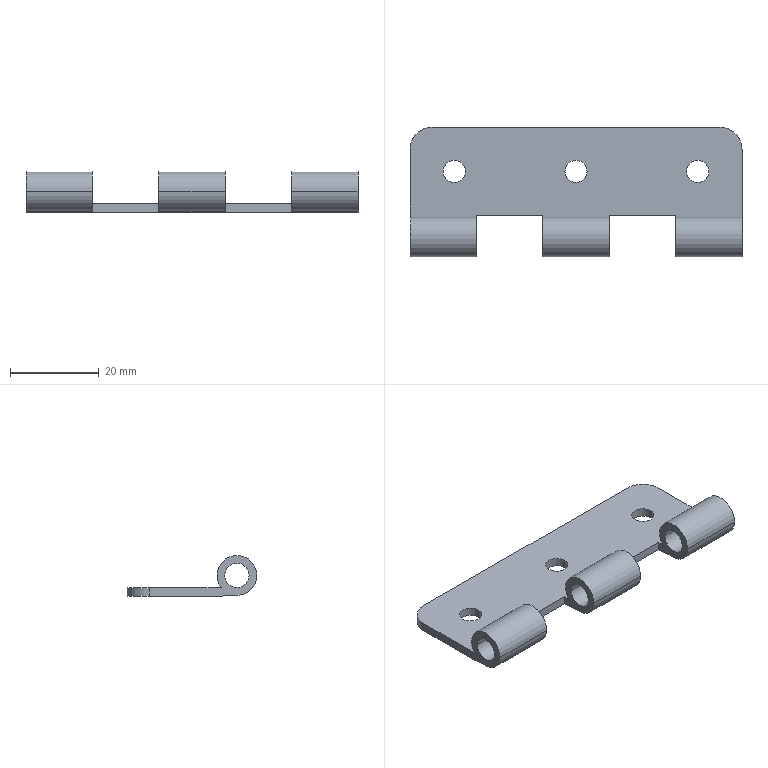Part | SolidWorks | features Extrusion 1, Fillet 1, ICE 1, LPattern 1 | 1 solid | 37 faces | box 75 x 29.3 x 9.25 mm | volume 4864 mm3 | cylinder 23 | plane 14 | commonest cylinder face diameters 9 x9 5 x6 5.5 x6 10 x2
STEP:
#1=CARTESIAN_POINT('',(75.,-22.05,4.75));
#2=VERTEX_POINT('',#1);
#3=CARTESIAN_POINT('',(75.,-27.55,4.75));
#4=VERTEX_POINT('',#3);
#5=CARTESIAN_POINT('',(75.,-24.8,4.75));
#6=DIRECTION('',(-1.,0.,0.));
#7=DIRECTION('',(0.,-1.,0.));
#8=AXIS2_PLACEMENT_3D('',#5,#6,#7);
#9=CIRCLE('',#8,2.75);
#10=EDGE_CURVE('',#2,#4,#9,.T.);
#11=ORIENTED_EDGE('',*,*,#10,.F.);
#12=CARTESIAN_POINT('',(60.,-22.05,4.75));
#13=VERTEX_POINT('',#12);
#14=CARTESIAN_POINT('',(75.,-22.05,4.75));
#15=DIRECTION('',(-1.,0.,0.));
#16=VECTOR('',#15,1000.);
#17=LINE('',#14,#16);
#18=EDGE_CURVE('',#2,#13,#17,.T.);
#19=ORIENTED_EDGE('',*,*,#18,.T.);
#20=CARTESIAN_POINT('',(60.,-27.55,4.75));
#21=VERTEX_POINT('',#20);
#22=CARTESIAN_POINT('',(60.,-24.8,4.75));
#23=DIRECTION('',(-1.,0.,0.));
#24=DIRECTION('',(0.,-1.,0.));
#25=AXIS2_PLACEMENT_3D('',#22,#23,#24);
#26=CIRCLE('',#25,2.75);
#27=EDGE_CURVE('',#13,#21,#26,.T.);
#28=ORIENTED_EDGE('',*,*,#27,.T.);
#29=CARTESIAN_POINT('',(75.,-27.55,4.75));
#30=DIRECTION('',(-1.,0.,0.));
#31=VECTOR('',#30,1000.);
#32=LINE('',#29,#31);
#33=EDGE_CURVE('',#4,#21,#32,.T.);
#34=ORIENTED_EDGE('',*,*,#33,.F.);
#35=EDGE_LOOP('',(#11,#19,#28,#34));
#36=FACE_OUTER_BOUND('',#35,.T.);
#37=CARTESIAN_POINT('',(75.,-24.8,4.75));
#38=DIRECTION('',(-1.,0.,0.));
#39=DIRECTION('',(0.,-1.,0.));
#40=AXIS2_PLACEMENT_3D('',#37,#38,#39);
#41=CYLINDRICAL_SURFACE('',#40,2.75);
#42=ADVANCED_FACE('',(#36),#41,.F.);
#43=CARTESIAN_POINT('',(75.,-29.3,4.75));
#44=VERTEX_POINT('',#43);
#45=CARTESIAN_POINT('',(75.,-20.3,4.75));
#46=VERTEX_POINT('',#45);
#47=CARTESIAN_POINT('',(75.,-24.8,4.75));
#48=DIRECTION('',(-1.,0.,0.));
#49=DIRECTION('',(0.,-1.,0.));
#50=AXIS2_PLACEMENT_3D('',#47,#48,#49);
#51=CIRCLE('',#50,4.5);
#52=EDGE_CURVE('',#44,#46,#51,.T.);
#53=ORIENTED_EDGE('',*,*,#52,.T.);
#54=CARTESIAN_POINT('',(60.,-20.3,4.75));
#55=VERTEX_POINT('',#54);
#56=CARTESIAN_POINT('',(75.,-20.3,4.75));
#57=DIRECTION('',(-1.,0.,0.));
#58=VECTOR('',#57,1000.);
#59=LINE('',#56,#58);
#60=EDGE_CURVE('',#46,#55,#59,.T.);
#61=ORIENTED_EDGE('',*,*,#60,.T.);
#62=CARTESIAN_POINT('',(60.,-29.3,4.75));
#63=VERTEX_POINT('',#62);
#64=CARTESIAN_POINT('',(60.,-24.8,4.75));
#65=DIRECTION('',(-1.,0.,0.));
#66=DIRECTION('',(0.,-1.,0.));
#67=AXIS2_PLACEMENT_3D('',#64,#65,#66);
#68=CIRCLE('',#67,4.5);
#69=EDGE_CURVE('',#63,#55,#68,.T.);
#70=ORIENTED_EDGE('',*,*,#69,.F.);
#71=CARTESIAN_POINT('',(75.,-29.3,4.75));
#72=DIRECTION('',(-1.,0.,0.));
#73=VECTOR('',#72,1000.);
#74=LINE('',#71,#73);
#75=EDGE_CURVE('',#44,#63,#74,.T.);
#76=ORIENTED_EDGE('',*,*,#75,.F.);
#77=EDGE_LOOP('',(#53,#61,#70,#76));
#78=FACE_OUTER_BOUND('',#77,.T.);
#79=CARTESIAN_POINT('',(75.,-24.8,4.75));
#80=DIRECTION('',(-1.,0.,0.));
#81=DIRECTION('',(0.,-1.,0.));
#82=AXIS2_PLACEMENT_3D('',#79,#80,#81);
#83=CYLINDRICAL_SURFACE('',#82,4.5);
#84=ADVANCED_FACE('',(#78),#83,.T.);
#85=CARTESIAN_POINT('',(75.,-25.029,0.2558));
#86=VERTEX_POINT('',#85);
#87=CARTESIAN_POINT('',(75.,-24.8,4.75));
#88=DIRECTION('',(-1.,0.,0.));
#89=DIRECTION('',(0.,-1.,0.));
#90=AXIS2_PLACEMENT_3D('',#87,#88,#89);
#91=CIRCLE('',#90,4.5);
#92=EDGE_CURVE('',#86,#44,#91,.T.);
#93=ORIENTED_EDGE('',*,*,#92,.T.);
#94=ORIENTED_EDGE('',*,*,#75,.T.);
#95=CARTESIAN_POINT('',(60.,-25.029,0.2558));
#96=VERTEX_POINT('',#95);
#97=CARTESIAN_POINT('',(60.,-24.8,4.75));
#98=DIRECTION('',(-1.,0.,0.));
#99=DIRECTION('',(0.,-1.,0.));
#100=AXIS2_PLACEMENT_3D('',#97,#98,#99);
#101=CIRCLE('',#100,4.5);
#102=EDGE_CURVE('',#96,#63,#101,.T.);
#103=ORIENTED_EDGE('',*,*,#102,.F.);
#104=CARTESIAN_POINT('',(75.,-25.029,0.2558));
#105=DIRECTION('',(-1.,0.,0.));
#106=VECTOR('',#105,1000.);
#107=LINE('',#104,#106);
#108=EDGE_CURVE('',#86,#96,#107,.T.);
#109=ORIENTED_EDGE('',*,*,#108,.F.);
#110=EDGE_LOOP('',(#93,#94,#103,#109));
#111=FACE_OUTER_BOUND('',#110,.T.);
#112=CARTESIAN_POINT('',(75.,-24.8,4.75));
#113=DIRECTION('',(-1.,0.,0.));
#114=DIRECTION('',(0.,-1.,0.));
#115=AXIS2_PLACEMENT_3D('',#112,#113,#114);
#116=CYLINDRICAL_SURFACE('',#115,4.5);
#117=ADVANCED_FACE('',(#111),#116,.T.);
#118=CARTESIAN_POINT('',(45.,-22.05,4.75));
#119=VERTEX_POINT('',#118);
#120=CARTESIAN_POINT('',(45.,-27.55,4.75));
#121=VERTEX_POINT('',#120);
#122=CARTESIAN_POINT('',(45.,-24.8,4.75));
#123=DIRECTION('',(-1.,0.,0.));
#124=DIRECTION('',(0.,-1.,0.));
#125=AXIS2_PLACEMENT_3D('',#122,#123,#124);
#126=CIRCLE('',#125,2.75);
#127=EDGE_CURVE('',#119,#121,#126,.T.);
#128=ORIENTED_EDGE('',*,*,#127,.F.);
#129=CARTESIAN_POINT('',(30.,-22.05,4.75));
#130=VERTEX_POINT('',#129);
#131=CARTESIAN_POINT('',(45.,-22.05,4.75));
#132=DIRECTION('',(-1.,0.,0.));
#133=VECTOR('',#132,1000.);
#134=LINE('',#131,#133);
#135=EDGE_CURVE('',#119,#130,#134,.T.);
#136=ORIENTED_EDGE('',*,*,#135,.T.);
#137=CARTESIAN_POINT('',(30.,-27.55,4.75));
#138=VERTEX_POINT('',#137);
#139=CARTESIAN_POINT('',(30.,-24.8,4.75));
#140=DIRECTION('',(-1.,0.,0.));
#141=DIRECTION('',(0.,-1.,0.));
#142=AXIS2_PLACEMENT_3D('',#139,#140,#141);
#143=CIRCLE('',#142,2.75);
#144=EDGE_CURVE('',#130,#138,#143,.T.);
#145=ORIENTED_EDGE('',*,*,#144,.T.);
#146=CARTESIAN_POINT('',(45.,-27.55,4.75));
#147=DIRECTION('',(-1.,0.,0.));
#148=VECTOR('',#147,1000.);
#149=LINE('',#146,#148);
#150=EDGE_CURVE('',#121,#138,#149,.T.);
#151=ORIENTED_EDGE('',*,*,#150,.F.);
#152=EDGE_LOOP('',(#128,#136,#145,#151));
#153=FACE_OUTER_BOUND('',#152,.T.);
#154=CARTESIAN_POINT('',(45.,-24.8,4.75));
#155=DIRECTION('',(-1.,0.,0.));
#156=DIRECTION('',(0.,-1.,0.));
#157=AXIS2_PLACEMENT_3D('',#154,#155,#156);
#158=CYLINDRICAL_SURFACE('',#157,2.75);
#159=ADVANCED_FACE('',(#153),#158,.F.);
#160=CARTESIAN_POINT('',(45.,-29.3,4.75));
#161=VERTEX_POINT('',#160);
#162=CARTESIAN_POINT('',(45.,-20.3,4.75));
#163=VERTEX_POINT('',#162);
#164=CARTESIAN_POINT('',(45.,-24.8,4.75));
#165=DIRECTION('',(-1.,0.,0.));
#166=DIRECTION('',(0.,-1.,0.));
#167=AXIS2_PLACEMENT_3D('',#164,#165,#166);
#168=CIRCLE('',#167,4.5);
#169=EDGE_CURVE('',#161,#163,#168,.T.);
#170=ORIENTED_EDGE('',*,*,#169,.T.);
#171=CARTESIAN_POINT('',(30.,-20.3,4.75));
#172=VERTEX_POINT('',#171);
#173=CARTESIAN_POINT('',(45.,-20.3,4.75));
#174=DIRECTION('',(-1.,0.,0.));
#175=VECTOR('',#174,1000.);
#176=LINE('',#173,#175);
#177=EDGE_CURVE('',#163,#172,#176,.T.);
#178=ORIENTED_EDGE('',*,*,#177,.T.);
#179=CARTESIAN_POINT('',(30.,-29.3,4.75));
#180=VERTEX_POINT('',#179);
#181=CARTESIAN_POINT('',(30.,-24.8,4.75));
#182=DIRECTION('',(-1.,0.,0.));
#183=DIRECTION('',(0.,-1.,0.));
#184=AXIS2_PLACEMENT_3D('',#181,#182,#183);
#185=CIRCLE('',#184,4.5);
#186=EDGE_CURVE('',#180,#172,#185,.T.);
#187=ORIENTED_EDGE('',*,*,#186,.F.);
#188=CARTESIAN_POINT('',(45.,-29.3,4.75));
#189=DIRECTION('',(-1.,0.,0.));
#190=VECTOR('',#189,1000.);
#191=LINE('',#188,#190);
#192=EDGE_CURVE('',#161,#180,#191,.T.);
#193=ORIENTED_EDGE('',*,*,#192,.F.);
#194=EDGE_LOOP('',(#170,#178,#187,#193));
#195=FACE_OUTER_BOUND('',#194,.T.);
#196=CARTESIAN_POINT('',(45.,-24.8,4.75));
#197=DIRECTION('',(-1.,0.,0.));
#198=DIRECTION('',(0.,-1.,0.));
#199=AXIS2_PLACEMENT_3D('',#196,#197,#198);
#200=CYLINDRICAL_SURFACE('',#199,4.5);
#201=ADVANCED_FACE('',(#195),#200,.T.);
#202=CARTESIAN_POINT('',(45.,-25.029,0.2558));
#203=VERTEX_POINT('',#202);
#204=CARTESIAN_POINT('',(45.,-24.8,4.75));
#205=DIRECTION('',(-1.,0.,0.));
#206=DIRECTION('',(0.,-1.,0.));
#207=AXIS2_PLACEMENT_3D('',#204,#205,#206);
#208=CIRCLE('',#207,4.5);
#209=EDGE_CURVE('',#203,#161,#208,.T.);
#210=ORIENTED_EDGE('',*,*,#209,.T.);
#211=ORIENTED_EDGE('',*,*,#192,.T.);
#212=CARTESIAN_POINT('',(30.,-25.029,0.2558));
#213=VERTEX_POINT('',#212);
#214=CARTESIAN_POINT('',(30.,-24.8,4.75));
#215=DIRECTION('',(-1.,0.,0.));
#216=DIRECTION('',(0.,-1.,0.));
#217=AXIS2_PLACEMENT_3D('',#214,#215,#216);
#218=CIRCLE('',#217,4.5);
#219=EDGE_CURVE('',#213,#180,#218,.T.);
#220=ORIENTED_EDGE('',*,*,#219,.F.);
#221=CARTESIAN_POINT('',(45.,-25.029,0.2558));
#222=DIRECTION('',(-1.,0.,0.));
#223=VECTOR('',#222,1000.);
#224=LINE('',#221,#223);
#225=EDGE_CURVE('',#203,#213,#224,.T.);
#226=ORIENTED_EDGE('',*,*,#225,.F.);
#227=EDGE_LOOP('',(#210,#211,#220,#226));
#228=FACE_OUTER_BOUND('',#227,.T.);
#229=CARTESIAN_POINT('',(45.,-24.8,4.75));
#230=DIRECTION('',(-1.,0.,0.));
#231=DIRECTION('',(0.,-1.,0.));
#232=AXIS2_PLACEMENT_3D('',#229,#230,#231);
#233=CYLINDRICAL_SURFACE('',#232,4.5);
#234=ADVANCED_FACE('',(#228),#233,.T.);
#235=CARTESIAN_POINT('',(15.,-22.05,4.75));
#236=VERTEX_POINT('',#235);
#237=CARTESIAN_POINT('',(15.,-27.55,4.75));
#238=VERTEX_POINT('',#237);
#239=CARTESIAN_POINT('',(15.,-24.8,4.75));
#240=DIRECTION('',(-1.,0.,0.));
#241=DIRECTION('',(0.,-1.,0.));
#242=AXIS2_PLACEMENT_3D('',#239,#240,#241);
#243=CIRCLE('',#242,2.75);
#244=EDGE_CURVE('',#236,#238,#243,.T.);
#245=ORIENTED_EDGE('',*,*,#244,.F.);
#246=CARTESIAN_POINT('',(0.,-22.05,4.75));
#247=VERTEX_POINT('',#246);
#248=CARTESIAN_POINT('',(15.,-22.05,4.75));
#249=DIRECTION('',(-1.,0.,0.));
#250=VECTOR('',#249,1000.);
#251=LINE('',#248,#250);
#252=EDGE_CURVE('',#236,#247,#251,.T.);
#253=ORIENTED_EDGE('',*,*,#252,.T.);
#254=CARTESIAN_POINT('',(0.,-27.55,4.75));
#255=VERTEX_POINT('',#254);
#256=CARTESIAN_POINT('',(0.,-24.8,4.75));
#257=DIRECTION('',(-1.,0.,0.));
#258=DIRECTION('',(0.,-1.,0.));
#259=AXIS2_PLACEMENT_3D('',#256,#257,#258);
#260=CIRCLE('',#259,2.75);
#261=EDGE_CURVE('',#247,#255,#260,.T.);
#262=ORIENTED_EDGE('',*,*,#261,.T.);
#263=CARTESIAN_POINT('',(15.,-27.55,4.75));
#264=DIRECTION('',(-1.,0.,0.));
#265=VECTOR('',#264,1000.);
#266=LINE('',#263,#265);
#267=EDGE_CURVE('',#238,#255,#266,.T.);
#268=ORIENTED_EDGE('',*,*,#267,.F.);
#269=EDGE_LOOP('',(#245,#253,#262,#268));
#270=FACE_OUTER_BOUND('',#269,.T.);
#271=CARTESIAN_POINT('',(15.,-24.8,4.75));
#272=DIRECTION('',(-1.,0.,0.));
#273=DIRECTION('',(0.,-1.,0.));
#274=AXIS2_PLACEMENT_3D('',#271,#272,#273);
#275=CYLINDRICAL_SURFACE('',#274,2.75);
#276=ADVANCED_FACE('',(#270),#275,.F.);
#277=CARTESIAN_POINT('',(15.,-29.3,4.75));
#278=VERTEX_POINT('',#277);
#279=CARTESIAN_POINT('',(15.,-20.3,4.75));
#280=VERTEX_POINT('',#279);
#281=CARTESIAN_POINT('',(15.,-24.8,4.75));
#282=DIRECTION('',(-1.,0.,0.));
#283=DIRECTION('',(0.,-1.,0.));
#284=AXIS2_PLACEMENT_3D('',#281,#282,#283);
#285=CIRCLE('',#284,4.5);
#286=EDGE_CURVE('',#278,#280,#285,.T.);
#287=ORIENTED_EDGE('',*,*,#286,.T.);
#288=CARTESIAN_POINT('',(0.,-20.3,4.75));
#289=VERTEX_POINT('',#288);
#290=CARTESIAN_POINT('',(15.,-20.3,4.75));
#291=DIRECTION('',(-1.,0.,0.));
#292=VECTOR('',#291,1000.);
#293=LINE('',#290,#292);
#294=EDGE_CURVE('',#280,#289,#293,.T.);
#295=ORIENTED_EDGE('',*,*,#294,.T.);
#296=CARTESIAN_POINT('',(0.,-29.3,4.75));
#297=VERTEX_POINT('',#296);
#298=CARTESIAN_POINT('',(0.,-24.8,4.75));
#299=DIRECTION('',(-1.,0.,0.));
#300=DIRECTION('',(0.,-1.,0.));
#301=AXIS2_PLACEMENT_3D('',#298,#299,#300);
#302=CIRCLE('',#301,4.5);
#303=EDGE_CURVE('',#297,#289,#302,.T.);
#304=ORIENTED_EDGE('',*,*,#303,.F.);
#305=CARTESIAN_POINT('',(15.,-29.3,4.75));
#306=DIRECTION('',(-1.,0.,0.));
#307=VECTOR('',#306,1000.);
#308=LINE('',#305,#307);
#309=EDGE_CURVE('',#278,#297,#308,.T.);
#310=ORIENTED_EDGE('',*,*,#309,.F.);
#311=EDGE_LOOP('',(#287,#295,#304,#310));
#312=FACE_OUTER_BOUND('',#311,.T.);
#313=CARTESIAN_POINT('',(15.,-24.8,4.75));
#314=DIRECTION('',(-1.,0.,0.));
#315=DIRECTION('',(0.,-1.,0.));
#316=AXIS2_PLACEMENT_3D('',#313,#314,#315);
#317=CYLINDRICAL_SURFACE('',#316,4.5);
#318=ADVANCED_FACE('',(#312),#317,.T.);
#319=CARTESIAN_POINT('',(15.,-25.029,0.2558));
#320=VERTEX_POINT('',#319);
#321=CARTESIAN_POINT('',(15.,-24.8,4.75));
#322=DIRECTION('',(-1.,0.,0.));
#323=DIRECTION('',(0.,-1.,0.));
#324=AXIS2_PLACEMENT_3D('',#321,#322,#323);
#325=CIRCLE('',#324,4.5);
#326=EDGE_CURVE('',#320,#278,#325,.T.);
#327=ORIENTED_EDGE('',*,*,#326,.T.);
#328=ORIENTED_EDGE('',*,*,#309,.T.);
#329=CARTESIAN_POINT('',(0.,-25.029,0.2558));
#330=VERTEX_POINT('',#329);
#331=CARTESIAN_POINT('',(0.,-24.8,4.75));
#332=DIRECTION('',(-1.,0.,0.));
#333=DIRECTION('',(0.,-1.,0.));
#334=AXIS2_PLACEMENT_3D('',#331,#332,#333);
#335=CIRCLE('',#334,4.5);
#336=EDGE_CURVE('',#330,#297,#335,.T.);
#337=ORIENTED_EDGE('',*,*,#336,.F.);
#338=CARTESIAN_POINT('',(15.,-25.029,0.2558));
#339=DIRECTION('',(-1.,0.,0.));
#340=VECTOR('',#339,1000.);
#341=LINE('',#338,#340);
#342=EDGE_CURVE('',#320,#330,#341,.T.);
#343=ORIENTED_EDGE('',*,*,#342,.F.);
#344=EDGE_LOOP('',(#327,#328,#337,#343));
#345=FACE_OUTER_BOUND('',#344,.T.);
#346=CARTESIAN_POINT('',(15.,-24.8,4.75));
#347=DIRECTION('',(-1.,0.,0.));
#348=DIRECTION('',(0.,-1.,0.));
#349=AXIS2_PLACEMENT_3D('',#346,#347,#348);
#350=CYLINDRICAL_SURFACE('',#349,4.5);
#351=ADVANCED_FACE('',(#345),#350,.T.);
#352=CARTESIAN_POINT('',(35.,-10.,2.));
#353=VERTEX_POINT('',#352);
#354=CARTESIAN_POINT('',(40.,-10.,2.));
#355=VERTEX_POINT('',#354);
#356=CARTESIAN_POINT('',(37.5,-10.,2.));
#357=DIRECTION('',(0.,0.,1.));
#358=DIRECTION('',(1.,0.,0.));
#359=AXIS2_PLACEMENT_3D('',#356,#357,#358);
#360=CIRCLE('',#359,2.5);
#361=EDGE_CURVE('',#353,#355,#360,.T.);
#362=ORIENTED_EDGE('',*,*,#361,.T.);
#363=CARTESIAN_POINT('',(40.,-10.,0.));
#364=VERTEX_POINT('',#363);
#365=CARTESIAN_POINT('',(40.,-10.,2.));
#366=DIRECTION('',(0.,0.,-1.));
#367=VECTOR('',#366,1000.);
#368=LINE('',#365,#367);
#369=EDGE_CURVE('',#355,#364,#368,.T.);
#370=ORIENTED_EDGE('',*,*,#369,.T.);
#371=CARTESIAN_POINT('',(35.,-10.,0.));
#372=VERTEX_POINT('',#371);
#373=CARTESIAN_POINT('',(37.5,-10.,0.));
#374=DIRECTION('',(0.,0.,1.));
#375=DIRECTION('',(1.,0.,0.));
#376=AXIS2_PLACEMENT_3D('',#373,#374,#375);
#377=CIRCLE('',#376,2.5);
#378=EDGE_CURVE('',#372,#364,#377,.T.);
#379=ORIENTED_EDGE('',*,*,#378,.F.);
#380=CARTESIAN_POINT('',(35.,-10.,2.));
#381=DIRECTION('',(0.,0.,-1.));
#382=VECTOR('',#381,1000.);
#383=LINE('',#380,#382);
#384=EDGE_CURVE('',#353,#372,#383,.T.);
#385=ORIENTED_EDGE('',*,*,#384,.F.);
#386=EDGE_LOOP('',(#362,#370,#379,#385));
#387=FACE_OUTER_BOUND('',#386,.T.);
#388=CARTESIAN_POINT('',(37.5,-10.,2.));
#389=DIRECTION('',(0.,0.,-1.));
#390=DIRECTION('',(-1.,0.,0.));
#391=AXIS2_PLACEMENT_3D('',#388,#389,#390);
#392=CYLINDRICAL_SURFACE('',#391,2.5);
#393=ADVANCED_FACE('',(#387),#392,.F.);
#394=CARTESIAN_POINT('',(62.5,-10.,2.));
#395=VERTEX_POINT('',#394);
#396=CARTESIAN_POINT('',(67.5,-10.,2.));
#397=VERTEX_POINT('',#396);
#398=CARTESIAN_POINT('',(65.,-10.,2.));
#399=DIRECTION('',(0.,0.,1.));
#400=DIRECTION('',(1.,0.,0.));
#401=AXIS2_PLACEMENT_3D('',#398,#399,#400);
#402=CIRCLE('',#401,2.5);
#403=EDGE_CURVE('',#395,#397,#402,.T.);
#404=ORIENTED_EDGE('',*,*,#403,.T.);
#405=CARTESIAN_POINT('',(67.5,-10.,0.));
#406=VERTEX_POINT('',#405);
#407=CARTESIAN_POINT('',(67.5,-10.,2.));
#408=DIRECTION('',(0.,0.,-1.));
#409=VECTOR('',#408,1000.);
#410=LINE('',#407,#409);
#411=EDGE_CURVE('',#397,#406,#410,.T.);
#412=ORIENTED_EDGE('',*,*,#411,.T.);
#413=CARTESIAN_POINT('',(62.5,-10.,0.));
#414=VERTEX_POINT('',#413);
#415=CARTESIAN_POINT('',(65.,-10.,0.));
#416=DIRECTION('',(0.,0.,1.));
#417=DIRECTION('',(1.,0.,0.));
#418=AXIS2_PLACEMENT_3D('',#415,#416,#417);
#419=CIRCLE('',#418,2.5);
#420=EDGE_CURVE('',#414,#406,#419,.T.);
#421=ORIENTED_EDGE('',*,*,#420,.F.);
#422=CARTESIAN_POINT('',(62.5,-10.,2.));
#423=DIRECTION('',(0.,0.,-1.));
#424=VECTOR('',#423,1000.);
#425=LINE('',#422,#424);
#426=EDGE_CURVE('',#395,#414,#425,.T.);
#427=ORIENTED_EDGE('',*,*,#426,.F.);
#428=EDGE_LOOP('',(#404,#412,#421,#427));
#429=FACE_OUTER_BOUND('',#428,.T.);
#430=CARTESIAN_POINT('',(65.,-10.,2.));
#431=DIRECTION('',(0.,0.,-1.));
#432=DIRECTION('',(-1.,0.,0.));
#433=AXIS2_PLACEMENT_3D('',#430,#431,#432);
#434=CYLINDRICAL_SURFACE('',#433,2.5);
#435=ADVANCED_FACE('',(#429),#434,.F.);
#436=CARTESIAN_POINT('',(7.5,-10.,2.));
#437=VERTEX_POINT('',#436);
#438=CARTESIAN_POINT('',(12.5,-10.,2.));
#439=VERTEX_POINT('',#438);
#440=CARTESIAN_POINT('',(10.,-10.,2.));
#441=DIRECTION('',(0.,0.,1.));
#442=DIRECTION('',(1.,0.,0.));
#443=AXIS2_PLACEMENT_3D('',#440,#441,#442);
#444=CIRCLE('',#443,2.5);
#445=EDGE_CURVE('',#437,#439,#444,.T.);
#446=ORIENTED_EDGE('',*,*,#445,.T.);
#447=CARTESIAN_POINT('',(12.5,-10.,0.));
#448=VERTEX_POINT('',#447);
#449=CARTESIAN_POINT('',(12.5,-10.,2.));
#450=DIRECTION('',(0.,0.,-1.));
#451=VECTOR('',#450,1000.);
#452=LINE('',#449,#451);
#453=EDGE_CURVE('',#439,#448,#452,.T.);
#454=ORIENTED_EDGE('',*,*,#453,.T.);
#455=CARTESIAN_POINT('',(7.5,-10.,0.));
#456=VERTEX_POINT('',#455);
#457=CARTESIAN_POINT('',(10.,-10.,0.));
#458=DIRECTION('',(0.,0.,1.));
#459=DIRECTION('',(1.,0.,0.));
#460=AXIS2_PLACEMENT_3D('',#457,#458,#459);
#461=CIRCLE('',#460,2.5);
#462=EDGE_CURVE('',#456,#448,#461,.T.);
#463=ORIENTED_EDGE('',*,*,#462,.F.);
#464=CARTESIAN_POINT('',(7.5,-10.,2.));
#465=DIRECTION('',(0.,0.,-1.));
#466=VECTOR('',#465,1000.);
#467=LINE('',#464,#466);
#468=EDGE_CURVE('',#437,#456,#467,.T.);
#469=ORIENTED_EDGE('',*,*,#468,.F.);
#470=EDGE_LOOP('',(#446,#454,#463,#469));
#471=FACE_OUTER_BOUND('',#470,.T.);
#472=CARTESIAN_POINT('',(10.,-10.,2.));
#473=DIRECTION('',(0.,0.,-1.));
#474=DIRECTION('',(-1.,0.,0.));
#475=AXIS2_PLACEMENT_3D('',#472,#473,#474);
#476=CYLINDRICAL_SURFACE('',#475,2.5);
#477=ADVANCED_FACE('',(#471),#476,.F.);
#478=CARTESIAN_POINT('',(45.,-20.,0.));
#479=VERTEX_POINT('',#478);
#480=CARTESIAN_POINT('',(60.,-20.,0.));
#481=VERTEX_POINT('',#480);
#482=CARTESIAN_POINT('',(0.,-20.,0.));
#483=DIRECTION('',(1.,0.,0.));
#484=VECTOR('',#483,1000.);
#485=LINE('',#482,#484);
#486=EDGE_CURVE('',#479,#481,#485,.T.);
#487=ORIENTED_EDGE('',*,*,#486,.T.);
#488=CARTESIAN_POINT('',(60.,-20.,2.));
#489=VERTEX_POINT('',#488);
#490=CARTESIAN_POINT('',(60.,-20.,0.));
#491=DIRECTION('',(0.,0.,1.));
#492=VECTOR('',#491,1000.);
#493=LINE('',#490,#492);
#494=EDGE_CURVE('',#481,#489,#493,.T.);
#495=ORIENTED_EDGE('',*,*,#494,.T.);
#496=CARTESIAN_POINT('',(45.,-20.,2.));
#497=VERTEX_POINT('',#496);
#498=CARTESIAN_POINT('',(0.,-20.,2.));
#499=DIRECTION('',(1.,0.,0.));
#500=VECTOR('',#499,1000.);
#501=LINE('',#498,#500);
#502=EDGE_CURVE('',#497,#489,#501,.T.);
#503=ORIENTED_EDGE('',*,*,#502,.F.);
#504=CARTESIAN_POINT('',(45.,-20.,0.));
#505=DIRECTION('',(0.,0.,1.));
#506=VECTOR('',#505,1000.);
#507=LINE('',#504,#506);
#508=EDGE_CURVE('',#479,#497,#507,.T.);
#509=ORIENTED_EDGE('',*,*,#508,.F.);
#510=EDGE_LOOP('',(#487,#495,#503,#509));
#511=FACE_OUTER_BOUND('',#510,.T.);
#512=CARTESIAN_POINT('',(0.,-20.,2.));
#513=DIRECTION('',(0.,1.,0.));
#514=DIRECTION('',(0.,0.,1.));
#515=AXIS2_PLACEMENT_3D('',#512,#513,#514);
#516=PLANE('',#515);
#517=ADVANCED_FACE('',(#511),#516,.F.);
#518=CARTESIAN_POINT('',(15.,-20.,0.));
#519=VERTEX_POINT('',#518);
#520=CARTESIAN_POINT('',(30.,-20.,0.));
#521=VERTEX_POINT('',#520);
#522=CARTESIAN_POINT('',(0.,-20.,0.));
#523=DIRECTION('',(1.,0.,0.));
#524=VECTOR('',#523,1000.);
#525=LINE('',#522,#524);
#526=EDGE_CURVE('',#519,#521,#525,.T.);
#527=ORIENTED_EDGE('',*,*,#526,.T.);
#528=CARTESIAN_POINT('',(30.,-20.,2.));
#529=VERTEX_POINT('',#528);
#530=CARTESIAN_POINT('',(30.,-20.,0.));
#531=DIRECTION('',(0.,0.,1.));
#532=VECTOR('',#531,1000.);
#533=LINE('',#530,#532);
#534=EDGE_CURVE('',#521,#529,#533,.T.);
#535=ORIENTED_EDGE('',*,*,#534,.T.);
#536=CARTESIAN_POINT('',(15.,-20.,2.));
#537=VERTEX_POINT('',#536);
#538=CARTESIAN_POINT('',(0.,-20.,2.));
#539=DIRECTION('',(1.,0.,0.));
#540=VECTOR('',#539,1000.);
#541=LINE('',#538,#540);
#542=EDGE_CURVE('',#537,#529,#541,.T.);
#543=ORIENTED_EDGE('',*,*,#542,.F.);
#544=CARTESIAN_POINT('',(15.,-20.,0.));
#545=DIRECTION('',(0.,0.,1.));
#546=VECTOR('',#545,1000.);
#547=LINE('',#544,#546);
#548=EDGE_CURVE('',#519,#537,#547,.T.);
#549=ORIENTED_EDGE('',*,*,#548,.F.);
#550=EDGE_LOOP('',(#527,#535,#543,#549));
#551=FACE_OUTER_BOUND('',#550,.T.);
#552=CARTESIAN_POINT('',(0.,-20.,2.));
#553=DIRECTION('',(0.,1.,0.));
#554=DIRECTION('',(0.,0.,1.));
#555=AXIS2_PLACEMENT_3D('',#552,#553,#554);
#556=PLANE('',#555);
#557=ADVANCED_FACE('',(#551),#556,.F.);
#558=ORIENTED_EDGE('',*,*,#403,.F.);
#559=CARTESIAN_POINT('',(65.,-10.,2.));
#560=DIRECTION('',(0.,0.,1.));
#561=DIRECTION('',(1.,0.,0.));
#562=AXIS2_PLACEMENT_3D('',#559,#560,#561);
#563=CIRCLE('',#562,2.5);
#564=EDGE_CURVE('',#397,#395,#563,.T.);
#565=ORIENTED_EDGE('',*,*,#564,.F.);
#566=EDGE_LOOP('',(#558,#565));
#567=FACE_BOUND('',#566,.T.);
#568=CARTESIAN_POINT('',(75.,-21.238,2.));
#569=VERTEX_POINT('',#568);
#570=CARTESIAN_POINT('',(75.,-5.,2.));
#571=VERTEX_POINT('',#570);
#572=CARTESIAN_POINT('',(75.,0.,2.));
#573=DIRECTION('',(0.,1.,0.));
#574=VECTOR('',#573,1000.);
#575=LINE('',#572,#574);
#576=EDGE_CURVE('',#569,#571,#575,.T.);
#577=ORIENTED_EDGE('',*,*,#576,.T.);
#578=CARTESIAN_POINT('',(70.,0.,2.));
#579=VERTEX_POINT('',#578);
#580=CARTESIAN_POINT('',(70.,-5.,2.));
#581=DIRECTION('',(0.,0.,1.));
#582=DIRECTION('',(1.,0.,0.));
#583=AXIS2_PLACEMENT_3D('',#580,#581,#582);
#584=CIRCLE('',#583,5.);
#585=EDGE_CURVE('',#571,#579,#584,.T.);
#586=ORIENTED_EDGE('',*,*,#585,.T.);
#587=CARTESIAN_POINT('',(5.,0.,2.));
#588=VERTEX_POINT('',#587);
#589=CARTESIAN_POINT('',(0.,0.,2.));
#590=DIRECTION('',(-1.,0.,0.));
#591=VECTOR('',#590,1000.);
#592=LINE('',#589,#591);
#593=EDGE_CURVE('',#579,#588,#592,.T.);
#594=ORIENTED_EDGE('',*,*,#593,.T.);
#595=CARTESIAN_POINT('',(0.,-5.,2.));
#596=VERTEX_POINT('',#595);
#597=CARTESIAN_POINT('',(5.,-5.,2.));
#598=DIRECTION('',(0.,0.,1.));
#599=DIRECTION('',(1.,0.,0.));
#600=AXIS2_PLACEMENT_3D('',#597,#598,#599);
#601=CIRCLE('',#600,5.);
#602=EDGE_CURVE('',#588,#596,#601,.T.);
#603=ORIENTED_EDGE('',*,*,#602,.T.);
#604=CARTESIAN_POINT('',(0.,-21.238,2.));
#605=VERTEX_POINT('',#604);
#606=CARTESIAN_POINT('',(0.,0.,2.));
#607=DIRECTION('',(0.,-1.,0.));
#608=VECTOR('',#607,1000.);
#609=LINE('',#606,#608);
#610=EDGE_CURVE('',#596,#605,#609,.T.);
#611=ORIENTED_EDGE('',*,*,#610,.T.);
#612=CARTESIAN_POINT('',(15.,-21.238,2.));
#613=VERTEX_POINT('',#612);
#614=CARTESIAN_POINT('',(15.,-21.238,2.));
#615=DIRECTION('',(-1.,0.,0.));
#616=VECTOR('',#615,1000.);
#617=LINE('',#614,#616);
#618=EDGE_CURVE('',#613,#605,#617,.T.);
#619=ORIENTED_EDGE('',*,*,#618,.F.);
#620=CARTESIAN_POINT('',(15.,0.,2.));
#621=DIRECTION('',(0.,-1.,0.));
#622=VECTOR('',#621,1000.);
#623=LINE('',#620,#622);
#624=EDGE_CURVE('',#537,#613,#623,.T.);
#625=ORIENTED_EDGE('',*,*,#624,.F.);
#626=ORIENTED_EDGE('',*,*,#542,.T.);
#627=CARTESIAN_POINT('',(30.,-21.238,2.));
#628=VERTEX_POINT('',#627);
#629=CARTESIAN_POINT('',(30.,0.,2.));
#630=DIRECTION('',(0.,-1.,0.));
#631=VECTOR('',#630,1000.);
#632=LINE('',#629,#631);
#633=EDGE_CURVE('',#529,#628,#632,.T.);
#634=ORIENTED_EDGE('',*,*,#633,.T.);
#635=CARTESIAN_POINT('',(45.,-21.238,2.));
#636=VERTEX_POINT('',#635);
#637=CARTESIAN_POINT('',(45.,-21.238,2.));
#638=DIRECTION('',(-1.,0.,0.));
#639=VECTOR('',#638,1000.);
#640=LINE('',#637,#639);
#641=EDGE_CURVE('',#636,#628,#640,.T.);
#642=ORIENTED_EDGE('',*,*,#641,.F.);
#643=CARTESIAN_POINT('',(45.,0.,2.));
#644=DIRECTION('',(0.,-1.,0.));
#645=VECTOR('',#644,1000.);
#646=LINE('',#643,#645);
#647=EDGE_CURVE('',#497,#636,#646,.T.);
#648=ORIENTED_EDGE('',*,*,#647,.F.);
#649=ORIENTED_EDGE('',*,*,#502,.T.);
#650=CARTESIAN_POINT('',(60.,-21.238,2.));
#651=VERTEX_POINT('',#650);
#652=CARTESIAN_POINT('',(60.,0.,2.));
#653=DIRECTION('',(0.,-1.,0.));
#654=VECTOR('',#653,1000.);
#655=LINE('',#652,#654);
#656=EDGE_CURVE('',#489,#651,#655,.T.);
#657=ORIENTED_EDGE('',*,*,#656,.T.);
#658=CARTESIAN_POINT('',(75.,-21.238,2.));
#659=DIRECTION('',(-1.,0.,0.));
#660=VECTOR('',#659,1000.);
#661=LINE('',#658,#660);
#662=EDGE_CURVE('',#569,#651,#661,.T.);
#663=ORIENTED_EDGE('',*,*,#662,.F.);
#664=EDGE_LOOP('',(#577,#586,#594,#603,#611,#619,#625,#626,#634,#642,#648,#649,#657,#663));
#665=FACE_OUTER_BOUND('',#664,.T.);
#666=ORIENTED_EDGE('',*,*,#445,.F.);
#667=CARTESIAN_POINT('',(10.,-10.,2.));
#668=DIRECTION('',(0.,0.,1.));
#669=DIRECTION('',(1.,0.,0.));
#670=AXIS2_PLACEMENT_3D('',#667,#668,#669);
#671=CIRCLE('',#670,2.5);
#672=EDGE_CURVE('',#439,#437,#671,.T.);
#673=ORIENTED_EDGE('',*,*,#672,.F.);
#674=EDGE_LOOP('',(#666,#673));
#675=FACE_BOUND('',#674,.T.);
#676=ORIENTED_EDGE('',*,*,#361,.F.);
#677=CARTESIAN_POINT('',(37.5,-10.,2.));
#678=DIRECTION('',(0.,0.,1.));
#679=DIRECTION('',(1.,0.,0.));
#680=AXIS2_PLACEMENT_3D('',#677,#678,#679);
#681=CIRCLE('',#680,2.5);
#682=EDGE_CURVE('',#355,#353,#681,.T.);
#683=ORIENTED_EDGE('',*,*,#682,.F.);
#684=EDGE_LOOP('',(#676,#683));
#685=FACE_BOUND('',#684,.T.);
#686=CARTESIAN_POINT('',(0.,0.,2.));
#687=DIRECTION('',(0.,0.,1.));
#688=DIRECTION('',(1.,0.,0.));
#689=AXIS2_PLACEMENT_3D('',#686,#687,#688);
#690=PLANE('',#689);
#691=ADVANCED_FACE('',(#567,#665,#675,#685),#690,.T.);
#692=CARTESIAN_POINT('',(70.,0.,0.));
#693=VERTEX_POINT('',#692);
#694=CARTESIAN_POINT('',(5.,0.,0.));
#695=VERTEX_POINT('',#694);
#696=CARTESIAN_POINT('',(0.,0.,0.));
#697=DIRECTION('',(-1.,0.,0.));
#698=VECTOR('',#697,1000.);
#699=LINE('',#696,#698);
#700=EDGE_CURVE('',#693,#695,#699,.T.);
#701=ORIENTED_EDGE('',*,*,#700,.F.);
#702=CARTESIAN_POINT('',(75.,-5.,0.));
#703=VERTEX_POINT('',#702);
#704=CARTESIAN_POINT('',(70.,-5.,0.));
#705=DIRECTION('',(0.,0.,-1.));
#706=DIRECTION('',(1.,0.,0.));
#707=AXIS2_PLACEMENT_3D('',#704,#705,#706);
#708=CIRCLE('',#707,5.);
#709=EDGE_CURVE('',#693,#703,#708,.T.);
#710=ORIENTED_EDGE('',*,*,#709,.T.);
#711=CARTESIAN_POINT('',(75.,-20.,0.));
#712=VERTEX_POINT('',#711);
#713=CARTESIAN_POINT('',(75.,0.,0.));
#714=DIRECTION('',(0.,1.,0.));
#715=VECTOR('',#714,1000.);
#716=LINE('',#713,#715);
#717=EDGE_CURVE('',#712,#703,#716,.T.);
#718=ORIENTED_EDGE('',*,*,#717,.F.);
#719=CARTESIAN_POINT('',(75.,-20.,0.));
#720=DIRECTION('',(-1.,0.,0.));
#721=VECTOR('',#720,1000.);
#722=LINE('',#719,#721);
#723=EDGE_CURVE('',#712,#481,#722,.T.);
#724=ORIENTED_EDGE('',*,*,#723,.T.);
#725=ORIENTED_EDGE('',*,*,#486,.F.);
#726=CARTESIAN_POINT('',(45.,-20.,0.));
#727=DIRECTION('',(-1.,0.,0.));
#728=VECTOR('',#727,1000.);
#729=LINE('',#726,#728);
#730=EDGE_CURVE('',#479,#521,#729,.T.);
#731=ORIENTED_EDGE('',*,*,#730,.T.);
#732=ORIENTED_EDGE('',*,*,#526,.F.);
#733=CARTESIAN_POINT('',(0.,-20.,0.));
#734=VERTEX_POINT('',#733);
#735=CARTESIAN_POINT('',(0.,-20.,0.));
#736=DIRECTION('',(1.,0.,0.));
#737=VECTOR('',#736,1000.);
#738=LINE('',#735,#737);
#739=EDGE_CURVE('',#734,#519,#738,.T.);
#740=ORIENTED_EDGE('',*,*,#739,.F.);
#741=CARTESIAN_POINT('',(0.,-5.,0.));
#742=VERTEX_POINT('',#741);
#743=CARTESIAN_POINT('',(0.,0.,0.));
#744=DIRECTION('',(0.,-1.,0.));
#745=VECTOR('',#744,1000.);
#746=LINE('',#743,#745);
#747=EDGE_CURVE('',#742,#734,#746,.T.);
#748=ORIENTED_EDGE('',*,*,#747,.F.);
#749=CARTESIAN_POINT('',(5.,-5.,0.));
#750=DIRECTION('',(0.,0.,-1.));
#751=DIRECTION('',(1.,0.,0.));
#752=AXIS2_PLACEMENT_3D('',#749,#750,#751);
#753=CIRCLE('',#752,5.);
#754=EDGE_CURVE('',#742,#695,#753,.T.);
#755=ORIENTED_EDGE('',*,*,#754,.T.);
#756=EDGE_LOOP('',(#701,#710,#718,#724,#725,#731,#732,#740,#748,#755));
#757=FACE_OUTER_BOUND('',#756,.T.);
#758=ORIENTED_EDGE('',*,*,#462,.T.);
#759=CARTESIAN_POINT('',(10.,-10.,0.));
#760=DIRECTION('',(0.,0.,1.));
#761=DIRECTION('',(1.,0.,0.));
#762=AXIS2_PLACEMENT_3D('',#759,#760,#761);
#763=CIRCLE('',#762,2.5);
#764=EDGE_CURVE('',#448,#456,#763,.T.);
#765=ORIENTED_EDGE('',*,*,#764,.T.);
#766=EDGE_LOOP('',(#758,#765));
#767=FACE_BOUND('',#766,.T.);
#768=ORIENTED_EDGE('',*,*,#420,.T.);
#769=CARTESIAN_POINT('',(65.,-10.,0.));
#770=DIRECTION('',(0.,0.,1.));
#771=DIRECTION('',(1.,0.,0.));
#772=AXIS2_PLACEMENT_3D('',#769,#770,#771);
#773=CIRCLE('',#772,2.5);
#774=EDGE_CURVE('',#406,#414,#773,.T.);
#775=ORIENTED_EDGE('',*,*,#774,.T.);
#776=EDGE_LOOP('',(#768,#775));
#777=FACE_BOUND('',#776,.T.);
#778=ORIENTED_EDGE('',*,*,#378,.T.);
#779=CARTESIAN_POINT('',(37.5,-10.,0.));
#780=DIRECTION('',(0.,0.,1.));
#781=DIRECTION('',(1.,0.,0.));
#782=AXIS2_PLACEMENT_3D('',#779,#780,#781);
#783=CIRCLE('',#782,2.5);
#784=EDGE_CURVE('',#364,#372,#783,.T.);
#785=ORIENTED_EDGE('',*,*,#784,.T.);
#786=EDGE_LOOP('',(#778,#785));
#787=FACE_BOUND('',#786,.T.);
#788=CARTESIAN_POINT('',(0.,0.,0.));
#789=DIRECTION('',(0.,0.,1.));
#790=DIRECTION('',(1.,0.,0.));
#791=AXIS2_PLACEMENT_3D('',#788,#789,#790);
#792=PLANE('',#791);
#793=ADVANCED_FACE('',(#757,#767,#777,#787),#792,.F.);
#794=ORIENTED_EDGE('',*,*,#610,.F.);
#795=CARTESIAN_POINT('',(0.,-5.,2.));
#796=DIRECTION('',(0.,0.,-1.));
#797=VECTOR('',#796,1000.);
#798=LINE('',#795,#797);
#799=EDGE_CURVE('',#596,#742,#798,.T.);
#800=ORIENTED_EDGE('',*,*,#799,.T.);
#801=ORIENTED_EDGE('',*,*,#747,.T.);
#802=CARTESIAN_POINT('',(0.,-0.05162,-1.015));
#803=DIRECTION('',(0.,-0.9987,0.05081));
#804=VECTOR('',#803,1000.);
#805=LINE('',#802,#804);
#806=EDGE_CURVE('',#734,#330,#805,.T.);
#807=ORIENTED_EDGE('',*,*,#806,.T.);
#808=ORIENTED_EDGE('',*,*,#336,.T.);
#809=ORIENTED_EDGE('',*,*,#303,.T.);
#810=CARTESIAN_POINT('',(0.,-24.8,4.75));
#811=DIRECTION('',(-1.,0.,0.));
#812=DIRECTION('',(0.,-1.,0.));
#813=AXIS2_PLACEMENT_3D('',#810,#811,#812);
#814=CIRCLE('',#813,4.5);
#815=EDGE_CURVE('',#289,#605,#814,.T.);
#816=ORIENTED_EDGE('',*,*,#815,.T.);
#817=EDGE_LOOP('',(#794,#800,#801,#807,#808,#809,#816));
#818=FACE_OUTER_BOUND('',#817,.T.);
#819=CARTESIAN_POINT('',(0.,-24.8,4.75));
#820=DIRECTION('',(-1.,0.,0.));
#821=DIRECTION('',(0.,-1.,0.));
#822=AXIS2_PLACEMENT_3D('',#819,#820,#821);
#823=CIRCLE('',#822,2.75);
#824=EDGE_CURVE('',#255,#247,#823,.T.);
#825=ORIENTED_EDGE('',*,*,#824,.F.);
#826=ORIENTED_EDGE('',*,*,#261,.F.);
#827=EDGE_LOOP('',(#825,#826));
#828=FACE_BOUND('',#827,.T.);
#829=CARTESIAN_POINT('',(0.,0.,2.));
#830=DIRECTION('',(1.,0.,0.));
#831=DIRECTION('',(0.,1.,0.));
#832=AXIS2_PLACEMENT_3D('',#829,#830,#831);
#833=PLANE('',#832);
#834=ADVANCED_FACE('',(#818,#828),#833,.F.);
#835=ORIENTED_EDGE('',*,*,#717,.T.);
#836=CARTESIAN_POINT('',(75.,-5.,2.));
#837=DIRECTION('',(0.,0.,1.));
#838=VECTOR('',#837,1000.);
#839=LINE('',#836,#838);
#840=EDGE_CURVE('',#703,#571,#839,.T.);
#841=ORIENTED_EDGE('',*,*,#840,.T.);
#842=ORIENTED_EDGE('',*,*,#576,.F.);
#843=CARTESIAN_POINT('',(75.,-24.8,4.75));
#844=DIRECTION('',(-1.,0.,0.));
#845=DIRECTION('',(0.,-1.,0.));
#846=AXIS2_PLACEMENT_3D('',#843,#844,#845);
#847=CIRCLE('',#846,4.5);
#848=EDGE_CURVE('',#46,#569,#847,.T.);
#849=ORIENTED_EDGE('',*,*,#848,.F.);
#850=ORIENTED_EDGE('',*,*,#52,.F.);
#851=ORIENTED_EDGE('',*,*,#92,.F.);
#852=CARTESIAN_POINT('',(75.,-0.05162,-1.015));
#853=DIRECTION('',(0.,-0.9987,0.05081));
#854=VECTOR('',#853,1000.);
#855=LINE('',#852,#854);
#856=EDGE_CURVE('',#712,#86,#855,.T.);
#857=ORIENTED_EDGE('',*,*,#856,.F.);
#858=EDGE_LOOP('',(#835,#841,#842,#849,#850,#851,#857));
#859=FACE_OUTER_BOUND('',#858,.T.);
#860=CARTESIAN_POINT('',(75.,-24.8,4.75));
#861=DIRECTION('',(-1.,0.,0.));
#862=DIRECTION('',(0.,-1.,0.));
#863=AXIS2_PLACEMENT_3D('',#860,#861,#862);
#864=CIRCLE('',#863,2.75);
#865=EDGE_CURVE('',#4,#2,#864,.T.);
#866=ORIENTED_EDGE('',*,*,#865,.T.);
#867=ORIENTED_EDGE('',*,*,#10,.T.);
#868=EDGE_LOOP('',(#866,#867));
#869=FACE_BOUND('',#868,.T.);
#870=CARTESIAN_POINT('',(75.,0.,2.));
#871=DIRECTION('',(-1.,0.,0.));
#872=DIRECTION('',(0.,0.,1.));
#873=AXIS2_PLACEMENT_3D('',#870,#871,#872);
#874=PLANE('',#873);
#875=ADVANCED_FACE('',(#859,#869),#874,.F.);
#876=ORIENTED_EDGE('',*,*,#593,.F.);
#877=CARTESIAN_POINT('',(70.,0.,2.));
#878=DIRECTION('',(0.,0.,-1.));
#879=VECTOR('',#878,1000.);
#880=LINE('',#877,#879);
#881=EDGE_CURVE('',#579,#693,#880,.T.);
#882=ORIENTED_EDGE('',*,*,#881,.T.);
#883=ORIENTED_EDGE('',*,*,#700,.T.);
#884=CARTESIAN_POINT('',(5.,0.,2.));
#885=DIRECTION('',(0.,0.,1.));
#886=VECTOR('',#885,1000.);
#887=LINE('',#884,#886);
#888=EDGE_CURVE('',#695,#588,#887,.T.);
#889=ORIENTED_EDGE('',*,*,#888,.T.);
#890=EDGE_LOOP('',(#876,#882,#883,#889));
#891=FACE_OUTER_BOUND('',#890,.T.);
#892=CARTESIAN_POINT('',(0.,0.,2.));
#893=DIRECTION('',(0.,-1.,0.));
#894=DIRECTION('',(0.,0.,-1.));
#895=AXIS2_PLACEMENT_3D('',#892,#893,#894);
#896=PLANE('',#895);
#897=ADVANCED_FACE('',(#891),#896,.F.);
#898=ORIENTED_EDGE('',*,*,#453,.F.);
#899=ORIENTED_EDGE('',*,*,#672,.T.);
#900=ORIENTED_EDGE('',*,*,#468,.T.);
#901=ORIENTED_EDGE('',*,*,#764,.F.);
#902=EDGE_LOOP('',(#898,#899,#900,#901));
#903=FACE_OUTER_BOUND('',#902,.T.);
#904=CARTESIAN_POINT('',(10.,-10.,2.));
#905=DIRECTION('',(0.,0.,-1.));
#906=DIRECTION('',(-1.,0.,0.));
#907=AXIS2_PLACEMENT_3D('',#904,#905,#906);
#908=CYLINDRICAL_SURFACE('',#907,2.5);
#909=ADVANCED_FACE('',(#903),#908,.F.);
#910=ORIENTED_EDGE('',*,*,#411,.F.);
#911=ORIENTED_EDGE('',*,*,#564,.T.);
#912=ORIENTED_EDGE('',*,*,#426,.T.);
#913=ORIENTED_EDGE('',*,*,#774,.F.);
#914=EDGE_LOOP('',(#910,#911,#912,#913));
#915=FACE_OUTER_BOUND('',#914,.T.);
#916=CARTESIAN_POINT('',(65.,-10.,2.));
#917=DIRECTION('',(0.,0.,-1.));
#918=DIRECTION('',(-1.,0.,0.));
#919=AXIS2_PLACEMENT_3D('',#916,#917,#918);
#920=CYLINDRICAL_SURFACE('',#919,2.5);
#921=ADVANCED_FACE('',(#915),#920,.F.);
#922=ORIENTED_EDGE('',*,*,#369,.F.);
#923=ORIENTED_EDGE('',*,*,#682,.T.);
#924=ORIENTED_EDGE('',*,*,#384,.T.);
#925=ORIENTED_EDGE('',*,*,#784,.F.);
#926=EDGE_LOOP('',(#922,#923,#924,#925));
#927=FACE_OUTER_BOUND('',#926,.T.);
#928=CARTESIAN_POINT('',(37.5,-10.,2.));
#929=DIRECTION('',(0.,0.,-1.));
#930=DIRECTION('',(-1.,0.,0.));
#931=AXIS2_PLACEMENT_3D('',#928,#929,#930);
#932=CYLINDRICAL_SURFACE('',#931,2.5);
#933=ADVANCED_FACE('',(#927),#932,.F.);
#934=ORIENTED_EDGE('',*,*,#294,.F.);
#935=CARTESIAN_POINT('',(15.,-24.8,4.75));
#936=DIRECTION('',(-1.,0.,0.));
#937=DIRECTION('',(0.,-1.,0.));
#938=AXIS2_PLACEMENT_3D('',#935,#936,#937);
#939=CIRCLE('',#938,4.5);
#940=EDGE_CURVE('',#280,#613,#939,.T.);
#941=ORIENTED_EDGE('',*,*,#940,.T.);
#942=ORIENTED_EDGE('',*,*,#618,.T.);
#943=ORIENTED_EDGE('',*,*,#815,.F.);
#944=EDGE_LOOP('',(#934,#941,#942,#943));
#945=FACE_OUTER_BOUND('',#944,.T.);
#946=CARTESIAN_POINT('',(15.,-24.8,4.75));
#947=DIRECTION('',(-1.,0.,0.));
#948=DIRECTION('',(0.,-1.,0.));
#949=AXIS2_PLACEMENT_3D('',#946,#947,#948);
#950=CYLINDRICAL_SURFACE('',#949,4.5);
#951=ADVANCED_FACE('',(#945),#950,.T.);
#952=ORIENTED_EDGE('',*,*,#806,.F.);
#953=ORIENTED_EDGE('',*,*,#739,.T.);
#954=CARTESIAN_POINT('',(15.,-0.05162,-1.015));
#955=DIRECTION('',(0.,-0.9987,0.05081));
#956=VECTOR('',#955,1000.);
#957=LINE('',#954,#956);
#958=EDGE_CURVE('',#519,#320,#957,.T.);
#959=ORIENTED_EDGE('',*,*,#958,.T.);
#960=ORIENTED_EDGE('',*,*,#342,.T.);
#961=EDGE_LOOP('',(#952,#953,#959,#960));
#962=FACE_OUTER_BOUND('',#961,.T.);
#963=CARTESIAN_POINT('',(15.,-0.05162,-1.015));
#964=DIRECTION('',(0.,-0.05081,-0.9987));
#965=DIRECTION('',(0.,0.9987,-0.05081));
#966=AXIS2_PLACEMENT_3D('',#963,#964,#965);
#967=PLANE('',#966);
#968=ADVANCED_FACE('',(#962),#967,.T.);
#969=ORIENTED_EDGE('',*,*,#252,.F.);
#970=CARTESIAN_POINT('',(15.,-24.8,4.75));
#971=DIRECTION('',(-1.,0.,0.));
#972=DIRECTION('',(0.,-1.,0.));
#973=AXIS2_PLACEMENT_3D('',#970,#971,#972);
#974=CIRCLE('',#973,2.75);
#975=EDGE_CURVE('',#238,#236,#974,.T.);
#976=ORIENTED_EDGE('',*,*,#975,.F.);
#977=ORIENTED_EDGE('',*,*,#267,.T.);
#978=ORIENTED_EDGE('',*,*,#824,.T.);
#979=EDGE_LOOP('',(#969,#976,#977,#978));
#980=FACE_OUTER_BOUND('',#979,.T.);
#981=CARTESIAN_POINT('',(15.,-24.8,4.75));
#982=DIRECTION('',(-1.,0.,0.));
#983=DIRECTION('',(0.,-1.,0.));
#984=AXIS2_PLACEMENT_3D('',#981,#982,#983);
#985=CYLINDRICAL_SURFACE('',#984,2.75);
#986=ADVANCED_FACE('',(#980),#985,.F.);
#987=ORIENTED_EDGE('',*,*,#975,.T.);
#988=ORIENTED_EDGE('',*,*,#244,.T.);
#989=EDGE_LOOP('',(#987,#988));
#990=FACE_BOUND('',#989,.T.);
#991=ORIENTED_EDGE('',*,*,#326,.F.);
#992=ORIENTED_EDGE('',*,*,#958,.F.);
#993=ORIENTED_EDGE('',*,*,#548,.T.);
#994=ORIENTED_EDGE('',*,*,#624,.T.);
#995=ORIENTED_EDGE('',*,*,#940,.F.);
#996=ORIENTED_EDGE('',*,*,#286,.F.);
#997=EDGE_LOOP('',(#991,#992,#993,#994,#995,#996));
#998=FACE_OUTER_BOUND('',#997,.T.);
#999=CARTESIAN_POINT('',(15.,0.,0.));
#1000=DIRECTION('',(-1.,0.,0.));
#1001=DIRECTION('',(0.,-1.,0.));
#1002=AXIS2_PLACEMENT_3D('',#999,#1000,#1001);
#1003=PLANE('',#1002);
#1004=ADVANCED_FACE('',(#990,#998),#1003,.F.);
#1005=ORIENTED_EDGE('',*,*,#177,.F.);
#1006=CARTESIAN_POINT('',(45.,-24.8,4.75));
#1007=DIRECTION('',(-1.,0.,0.));
#1008=DIRECTION('',(0.,-1.,0.));
#1009=AXIS2_PLACEMENT_3D('',#1006,#1007,#1008);
#1010=CIRCLE('',#1009,4.5);
#1011=EDGE_CURVE('',#163,#636,#1010,.T.);
#1012=ORIENTED_EDGE('',*,*,#1011,.T.);
#1013=ORIENTED_EDGE('',*,*,#641,.T.);
#1014=CARTESIAN_POINT('',(30.,-24.8,4.75));
#1015=DIRECTION('',(-1.,0.,0.));
#1016=DIRECTION('',(0.,-1.,0.));
#1017=AXIS2_PLACEMENT_3D('',#1014,#1015,#1016);
#1018=CIRCLE('',#1017,4.5);
#1019=EDGE_CURVE('',#172,#628,#1018,.T.);
#1020=ORIENTED_EDGE('',*,*,#1019,.F.);
#1021=EDGE_LOOP('',(#1005,#1012,#1013,#1020));
#1022=FACE_OUTER_BOUND('',#1021,.T.);
#1023=CARTESIAN_POINT('',(45.,-24.8,4.75));
#1024=DIRECTION('',(-1.,0.,0.));
#1025=DIRECTION('',(0.,-1.,0.));
#1026=AXIS2_PLACEMENT_3D('',#1023,#1024,#1025);
#1027=CYLINDRICAL_SURFACE('',#1026,4.5);
#1028=ADVANCED_FACE('',(#1022),#1027,.T.);
#1029=CARTESIAN_POINT('',(30.,-0.05162,-1.015));
#1030=DIRECTION('',(0.,-0.9987,0.05081));
#1031=VECTOR('',#1030,1000.);
#1032=LINE('',#1029,#1031);
#1033=EDGE_CURVE('',#521,#213,#1032,.T.);
#1034=ORIENTED_EDGE('',*,*,#1033,.F.);
#1035=ORIENTED_EDGE('',*,*,#730,.F.);
#1036=CARTESIAN_POINT('',(45.,-0.05162,-1.015));
#1037=DIRECTION('',(0.,-0.9987,0.05081));
#1038=VECTOR('',#1037,1000.);
#1039=LINE('',#1036,#1038);
#1040=EDGE_CURVE('',#479,#203,#1039,.T.);
#1041=ORIENTED_EDGE('',*,*,#1040,.T.);
#1042=ORIENTED_EDGE('',*,*,#225,.T.);
#1043=EDGE_LOOP('',(#1034,#1035,#1041,#1042));
#1044=FACE_OUTER_BOUND('',#1043,.T.);
#1045=CARTESIAN_POINT('',(45.,-0.05162,-1.015));
#1046=DIRECTION('',(0.,-0.05081,-0.9987));
#1047=DIRECTION('',(0.,0.9987,-0.05081));
#1048=AXIS2_PLACEMENT_3D('',#1045,#1046,#1047);
#1049=PLANE('',#1048);
#1050=ADVANCED_FACE('',(#1044),#1049,.T.);
#1051=ORIENTED_EDGE('',*,*,#135,.F.);
#1052=CARTESIAN_POINT('',(45.,-24.8,4.75));
#1053=DIRECTION('',(-1.,0.,0.));
#1054=DIRECTION('',(0.,-1.,0.));
#1055=AXIS2_PLACEMENT_3D('',#1052,#1053,#1054);
#1056=CIRCLE('',#1055,2.75);
#1057=EDGE_CURVE('',#121,#119,#1056,.T.);
#1058=ORIENTED_EDGE('',*,*,#1057,.F.);
#1059=ORIENTED_EDGE('',*,*,#150,.T.);
#1060=CARTESIAN_POINT('',(30.,-24.8,4.75));
#1061=DIRECTION('',(-1.,0.,0.));
#1062=DIRECTION('',(0.,-1.,0.));
#1063=AXIS2_PLACEMENT_3D('',#1060,#1061,#1062);
#1064=CIRCLE('',#1063,2.75);
#1065=EDGE_CURVE('',#138,#130,#1064,.T.);
#1066=ORIENTED_EDGE('',*,*,#1065,.T.);
#1067=EDGE_LOOP('',(#1051,#1058,#1059,#1066));
#1068=FACE_OUTER_BOUND('',#1067,.T.);
#1069=CARTESIAN_POINT('',(45.,-24.8,4.75));
#1070=DIRECTION('',(-1.,0.,0.));
#1071=DIRECTION('',(0.,-1.,0.));
#1072=AXIS2_PLACEMENT_3D('',#1069,#1070,#1071);
#1073=CYLINDRICAL_SURFACE('',#1072,2.75);
#1074=ADVANCED_FACE('',(#1068),#1073,.F.);
#1075=ORIENTED_EDGE('',*,*,#1057,.T.);
#1076=ORIENTED_EDGE('',*,*,#127,.T.);
#1077=EDGE_LOOP('',(#1075,#1076));
#1078=FACE_BOUND('',#1077,.T.);
#1079=ORIENTED_EDGE('',*,*,#209,.F.);
#1080=ORIENTED_EDGE('',*,*,#1040,.F.);
#1081=ORIENTED_EDGE('',*,*,#508,.T.);
#1082=ORIENTED_EDGE('',*,*,#647,.T.);
#1083=ORIENTED_EDGE('',*,*,#1011,.F.);
#1084=ORIENTED_EDGE('',*,*,#169,.F.);
#1085=EDGE_LOOP('',(#1079,#1080,#1081,#1082,#1083,#1084));
#1086=FACE_OUTER_BOUND('',#1085,.T.);
#1087=CARTESIAN_POINT('',(45.,0.,0.));
#1088=DIRECTION('',(-1.,0.,0.));
#1089=DIRECTION('',(0.,-1.,0.));
#1090=AXIS2_PLACEMENT_3D('',#1087,#1088,#1089);
#1091=PLANE('',#1090);
#1092=ADVANCED_FACE('',(#1078,#1086),#1091,.F.);
#1093=ORIENTED_EDGE('',*,*,#1065,.F.);
#1094=ORIENTED_EDGE('',*,*,#144,.F.);
#1095=EDGE_LOOP('',(#1093,#1094));
#1096=FACE_BOUND('',#1095,.T.);
#1097=ORIENTED_EDGE('',*,*,#219,.T.);
#1098=ORIENTED_EDGE('',*,*,#186,.T.);
#1099=ORIENTED_EDGE('',*,*,#1019,.T.);
#1100=ORIENTED_EDGE('',*,*,#633,.F.);
#1101=ORIENTED_EDGE('',*,*,#534,.F.);
#1102=ORIENTED_EDGE('',*,*,#1033,.T.);
#1103=EDGE_LOOP('',(#1097,#1098,#1099,#1100,#1101,#1102));
#1104=FACE_OUTER_BOUND('',#1103,.T.);
#1105=CARTESIAN_POINT('',(30.,0.,0.));
#1106=DIRECTION('',(-1.,0.,0.));
#1107=DIRECTION('',(0.,-1.,0.));
#1108=AXIS2_PLACEMENT_3D('',#1105,#1106,#1107);
#1109=PLANE('',#1108);
#1110=ADVANCED_FACE('',(#1096,#1104),#1109,.T.);
#1111=ORIENTED_EDGE('',*,*,#60,.F.);
#1112=ORIENTED_EDGE('',*,*,#848,.T.);
#1113=ORIENTED_EDGE('',*,*,#662,.T.);
#1114=CARTESIAN_POINT('',(60.,-24.8,4.75));
#1115=DIRECTION('',(-1.,0.,0.));
#1116=DIRECTION('',(0.,-1.,0.));
#1117=AXIS2_PLACEMENT_3D('',#1114,#1115,#1116);
#1118=CIRCLE('',#1117,4.5);
#1119=EDGE_CURVE('',#55,#651,#1118,.T.);
#1120=ORIENTED_EDGE('',*,*,#1119,.F.);
#1121=EDGE_LOOP('',(#1111,#1112,#1113,#1120));
#1122=FACE_OUTER_BOUND('',#1121,.T.);
#1123=CARTESIAN_POINT('',(75.,-24.8,4.75));
#1124=DIRECTION('',(-1.,0.,0.));
#1125=DIRECTION('',(0.,-1.,0.));
#1126=AXIS2_PLACEMENT_3D('',#1123,#1124,#1125);
#1127=CYLINDRICAL_SURFACE('',#1126,4.5);
#1128=ADVANCED_FACE('',(#1122),#1127,.T.);
#1129=CARTESIAN_POINT('',(60.,-0.05162,-1.015));
#1130=DIRECTION('',(0.,-0.9987,0.05081));
#1131=VECTOR('',#1130,1000.);
#1132=LINE('',#1129,#1131);
#1133=EDGE_CURVE('',#481,#96,#1132,.T.);
#1134=ORIENTED_EDGE('',*,*,#1133,.F.);
#1135=ORIENTED_EDGE('',*,*,#723,.F.);
#1136=ORIENTED_EDGE('',*,*,#856,.T.);
#1137=ORIENTED_EDGE('',*,*,#108,.T.);
#1138=EDGE_LOOP('',(#1134,#1135,#1136,#1137));
#1139=FACE_OUTER_BOUND('',#1138,.T.);
#1140=CARTESIAN_POINT('',(75.,-0.05162,-1.015));
#1141=DIRECTION('',(0.,-0.05081,-0.9987));
#1142=DIRECTION('',(0.,0.9987,-0.05081));
#1143=AXIS2_PLACEMENT_3D('',#1140,#1141,#1142);
#1144=PLANE('',#1143);
#1145=ADVANCED_FACE('',(#1139),#1144,.T.);
#1146=ORIENTED_EDGE('',*,*,#18,.F.);
#1147=ORIENTED_EDGE('',*,*,#865,.F.);
#1148=ORIENTED_EDGE('',*,*,#33,.T.);
#1149=CARTESIAN_POINT('',(60.,-24.8,4.75));
#1150=DIRECTION('',(-1.,0.,0.));
#1151=DIRECTION('',(0.,-1.,0.));
#1152=AXIS2_PLACEMENT_3D('',#1149,#1150,#1151);
#1153=CIRCLE('',#1152,2.75);
#1154=EDGE_CURVE('',#21,#13,#1153,.T.);
#1155=ORIENTED_EDGE('',*,*,#1154,.T.);
#1156=EDGE_LOOP('',(#1146,#1147,#1148,#1155));
#1157=FACE_OUTER_BOUND('',#1156,.T.);
#1158=CARTESIAN_POINT('',(75.,-24.8,4.75));
#1159=DIRECTION('',(-1.,0.,0.));
#1160=DIRECTION('',(0.,-1.,0.));
#1161=AXIS2_PLACEMENT_3D('',#1158,#1159,#1160);
#1162=CYLINDRICAL_SURFACE('',#1161,2.75);
#1163=ADVANCED_FACE('',(#1157),#1162,.F.);
#1164=ORIENTED_EDGE('',*,*,#1154,.F.);
#1165=ORIENTED_EDGE('',*,*,#27,.F.);
#1166=EDGE_LOOP('',(#1164,#1165));
#1167=FACE_BOUND('',#1166,.T.);
#1168=ORIENTED_EDGE('',*,*,#102,.T.);
#1169=ORIENTED_EDGE('',*,*,#69,.T.);
#1170=ORIENTED_EDGE('',*,*,#1119,.T.);
#1171=ORIENTED_EDGE('',*,*,#656,.F.);
#1172=ORIENTED_EDGE('',*,*,#494,.F.);
#1173=ORIENTED_EDGE('',*,*,#1133,.T.);
#1174=EDGE_LOOP('',(#1168,#1169,#1170,#1171,#1172,#1173));
#1175=FACE_OUTER_BOUND('',#1174,.T.);
#1176=CARTESIAN_POINT('',(60.,0.,0.));
#1177=DIRECTION('',(-1.,0.,0.));
#1178=DIRECTION('',(0.,-1.,0.));
#1179=AXIS2_PLACEMENT_3D('',#1176,#1177,#1178);
#1180=PLANE('',#1179);
#1181=ADVANCED_FACE('',(#1167,#1175),#1180,.T.);
#1182=ORIENTED_EDGE('',*,*,#585,.F.);
#1183=ORIENTED_EDGE('',*,*,#840,.F.);
#1184=ORIENTED_EDGE('',*,*,#709,.F.);
#1185=ORIENTED_EDGE('',*,*,#881,.F.);
#1186=EDGE_LOOP('',(#1182,#1183,#1184,#1185));
#1187=FACE_OUTER_BOUND('',#1186,.T.);
#1188=CARTESIAN_POINT('',(70.,-5.,2.));
#1189=DIRECTION('',(0.,0.,-1.));
#1190=DIRECTION('',(-1.,0.,0.));
#1191=AXIS2_PLACEMENT_3D('',#1188,#1189,#1190);
#1192=CYLINDRICAL_SURFACE('',#1191,5.);
#1193=ADVANCED_FACE('',(#1187),#1192,.T.);
#1194=ORIENTED_EDGE('',*,*,#602,.F.);
#1195=ORIENTED_EDGE('',*,*,#888,.F.);
#1196=ORIENTED_EDGE('',*,*,#754,.F.);
#1197=ORIENTED_EDGE('',*,*,#799,.F.);
#1198=EDGE_LOOP('',(#1194,#1195,#1196,#1197));
#1199=FACE_OUTER_BOUND('',#1198,.T.);
#1200=CARTESIAN_POINT('',(5.,-5.,2.));
#1201=DIRECTION('',(0.,0.,-1.));
#1202=DIRECTION('',(-1.,0.,0.));
#1203=AXIS2_PLACEMENT_3D('',#1200,#1201,#1202);
#1204=CYLINDRICAL_SURFACE('',#1203,5.);
#1205=ADVANCED_FACE('',(#1199),#1204,.T.);
#1206=CLOSED_SHELL('',(#42,#84,#117,#159,#201,#234,#276,#318,#351,#393,#435,#477,#517,#557,#691,#793,#834,#875,#897,#909,#921,#933,#951,#968,#986,#1004,#1028,#1050,#1074,#1092,#1110,#1128,#1145,#1163,#1181,#1193,#1205));
#1207=MANIFOLD_SOLID_BREP('',#1206);
#1208=CARTESIAN_POINT('',(0.,0.,0.));
#1209=DIRECTION('',(0.,0.,1.));
#1210=DIRECTION('',(1.,0.,0.));
#1211=AXIS2_PLACEMENT_3D('',#1208,#1209,#1210);
#1212=(LENGTH_UNIT()NAMED_UNIT(*)SI_UNIT(.MILLI.,.METRE.));
#1213=UNCERTAINTY_MEASURE_WITH_UNIT(LENGTH_MEASURE(0.00001),#1212,'','');
#1214=(NAMED_UNIT(*)PLANE_ANGLE_UNIT()SI_UNIT($,.RADIAN.));
#1215=(NAMED_UNIT(*)SI_UNIT($,.STERADIAN.)SOLID_ANGLE_UNIT());
#1216=(GEOMETRIC_REPRESENTATION_CONTEXT(3)GLOBAL_UNCERTAINTY_ASSIGNED_CONTEXT((#1213))GLOBAL_UNIT_ASSIGNED_CONTEXT((#1212,#1214,#1215))REPRESENTATION_CONTEXT('',''));
#1217=ADVANCED_BREP_SHAPE_REPRESENTATION('',(#1207,#1211),#1216);